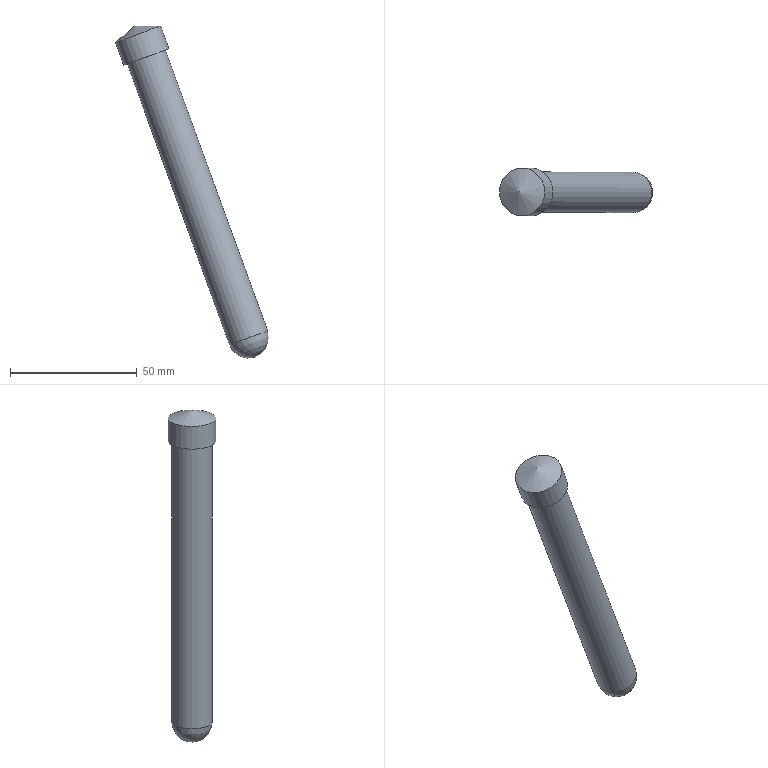Part | NX | features solid 2 | 1 solid | 5 faces | box 60.566 x 19 x 131.147 mm | volume 27840 mm3 | cylinder 2 | plane 1 | sphere 1 | cone 1 | commonest cylinder face diameters 16 x1 19 x1
STEP:
#1=CARTESIAN_POINT('',(62.01,-50.,55.548));
#2=VERTEX_POINT('',#1);
#3=CARTESIAN_POINT('',(69.527,-50.,58.284));
#4=DIRECTION('',(0.342,0.,-0.9397));
#5=DIRECTION('',(-0.9397,0.,-0.342));
#6=AXIS2_PLACEMENT_3D('',#3,#4,#5);
#7=CIRCLE('',#6,8.);
#8=EDGE_CURVE('',#2,#2,#7,.T.);
#9=ORIENTED_EDGE('',*,*,#8,.F.);
#10=EDGE_LOOP('',(#9));
#11=FACE_BOUND('',#10,.T.);
#12=CARTESIAN_POINT('',(60.6,-50.,55.035));
#13=VERTEX_POINT('',#12);
#14=CARTESIAN_POINT('',(69.527,-50.,58.284));
#15=DIRECTION('',(-0.342,0.,0.9397));
#16=DIRECTION('',(-0.9397,0.,-0.342));
#17=AXIS2_PLACEMENT_3D('',#14,#15,#16);
#18=CIRCLE('',#17,9.5);
#19=EDGE_CURVE('',#13,#13,#18,.T.);
#20=ORIENTED_EDGE('',*,*,#19,.F.);
#21=EDGE_LOOP('',(#20));
#22=FACE_BOUND('',#21,.T.);
#23=CARTESIAN_POINT('',(69.527,-50.,58.284));
#24=DIRECTION('',(0.342,0.,-0.9397));
#25=DIRECTION('',(-0.9397,0.,-0.342));
#26=AXIS2_PLACEMENT_3D('',#23,#24,#25);
#27=PLANE('',#26);
#28=ADVANCED_FACE('',(#11,#22),#27,.T.);
#29=ORIENTED_EDGE('',*,*,#19,.T.);
#30=EDGE_LOOP('',(#29));
#31=FACE_BOUND('',#30,.T.);
#32=CARTESIAN_POINT('',(57.336,-50.,64.002));
#33=VERTEX_POINT('',#32);
#34=CARTESIAN_POINT('',(66.264,-50.,67.251));
#35=DIRECTION('',(0.342,0.,-0.9397));
#36=DIRECTION('',(-0.9397,0.,-0.342));
#37=AXIS2_PLACEMENT_3D('',#34,#35,#36);
#38=CIRCLE('',#37,9.5);
#39=EDGE_CURVE('',#33,#33,#38,.T.);
#40=ORIENTED_EDGE('',*,*,#39,.T.);
#41=EDGE_LOOP('',(#40));
#42=FACE_BOUND('',#41,.T.);
#43=CARTESIAN_POINT('',(66.264,-50.,67.251));
#44=DIRECTION('',(0.342,0.,-0.9397));
#45=DIRECTION('',(-0.9397,0.,-0.342));
#46=AXIS2_PLACEMENT_3D('',#43,#44,#45);
#47=CYLINDRICAL_SURFACE('',#46,9.5);
#48=ADVANCED_FACE('',(#31,#42),#47,.T.);
#49=CARTESIAN_POINT('',(102.385,-50.,-55.383));
#50=VERTEX_POINT('',#49);
#51=CARTESIAN_POINT('',(109.903,-50.,-52.647));
#52=DIRECTION('',(0.342,0.,-0.9397));
#53=DIRECTION('',(-0.9397,0.,-0.342));
#54=AXIS2_PLACEMENT_3D('',#51,#52,#53);
#55=CIRCLE('',#54,8.);
#56=EDGE_CURVE('',#50,#50,#55,.T.);
#57=ORIENTED_EDGE('',*,*,#56,.F.);
#58=EDGE_LOOP('',(#57));
#59=FACE_BOUND('',#58,.T.);
#60=ORIENTED_EDGE('',*,*,#8,.T.);
#61=EDGE_LOOP('',(#60));
#62=FACE_BOUND('',#61,.T.);
#63=CARTESIAN_POINT('',(69.527,-50.,58.284));
#64=DIRECTION('',(0.342,0.,-0.9397));
#65=DIRECTION('',(-0.9397,0.,-0.342));
#66=AXIS2_PLACEMENT_3D('',#63,#64,#65);
#67=CYLINDRICAL_SURFACE('',#66,8.);
#68=ADVANCED_FACE('',(#59,#62),#67,.T.);
#69=ORIENTED_EDGE('',*,*,#56,.T.);
#70=EDGE_LOOP('',(#69));
#71=FACE_BOUND('',#70,.T.);
#72=CARTESIAN_POINT('',(109.903,-50.,-52.647));
#73=DIRECTION('',(0.342,0.,-0.9397));
#74=DIRECTION('',(-0.9397,0.,-0.342));
#75=AXIS2_PLACEMENT_3D('',#72,#73,#74);
#76=SPHERICAL_SURFACE('',#75,8.);
#77=ADVANCED_FACE('',(#71),#76,.T.);
#78=ORIENTED_EDGE('',*,*,#39,.F.);
#79=EDGE_LOOP('',(#78));
#80=FACE_BOUND('',#79,.T.);
#81=CARTESIAN_POINT('',(65.081,-50.,70.5));
#82=VERTEX_POINT('',#81);
#83=VERTEX_LOOP('',#82);
#84=FACE_BOUND('',#83,.T.);
#85=CARTESIAN_POINT('',(65.081,-50.,70.5));
#86=DIRECTION('',(0.342,0.,-0.9397));
#87=DIRECTION('',(-0.9397,0.,-0.342));
#88=AXIS2_PLACEMENT_3D('',#85,#86,#87);
#89=CONICAL_SURFACE('',#88,0.,1.222);
#90=ADVANCED_FACE('',(#80,#84),#89,.T.);
#91=CLOSED_SHELL('',(#28,#48,#68,#77,#90));
#92=MANIFOLD_SOLID_BREP('',#91);
#93=(LENGTH_UNIT()NAMED_UNIT(*)SI_UNIT(.MILLI.,.METRE.));
#94=UNCERTAINTY_MEASURE_WITH_UNIT(LENGTH_MEASURE(0.00001),#93,'','');
#95=(NAMED_UNIT(*)PLANE_ANGLE_UNIT()SI_UNIT($,.RADIAN.));
#96=(NAMED_UNIT(*)SI_UNIT($,.STERADIAN.)SOLID_ANGLE_UNIT());
#97=(GEOMETRIC_REPRESENTATION_CONTEXT(3)GLOBAL_UNCERTAINTY_ASSIGNED_CONTEXT((#94))GLOBAL_UNIT_ASSIGNED_CONTEXT((#93,#95,#96))REPRESENTATION_CONTEXT('',''));
#98=ADVANCED_BREP_SHAPE_REPRESENTATION('',(#92),#97);